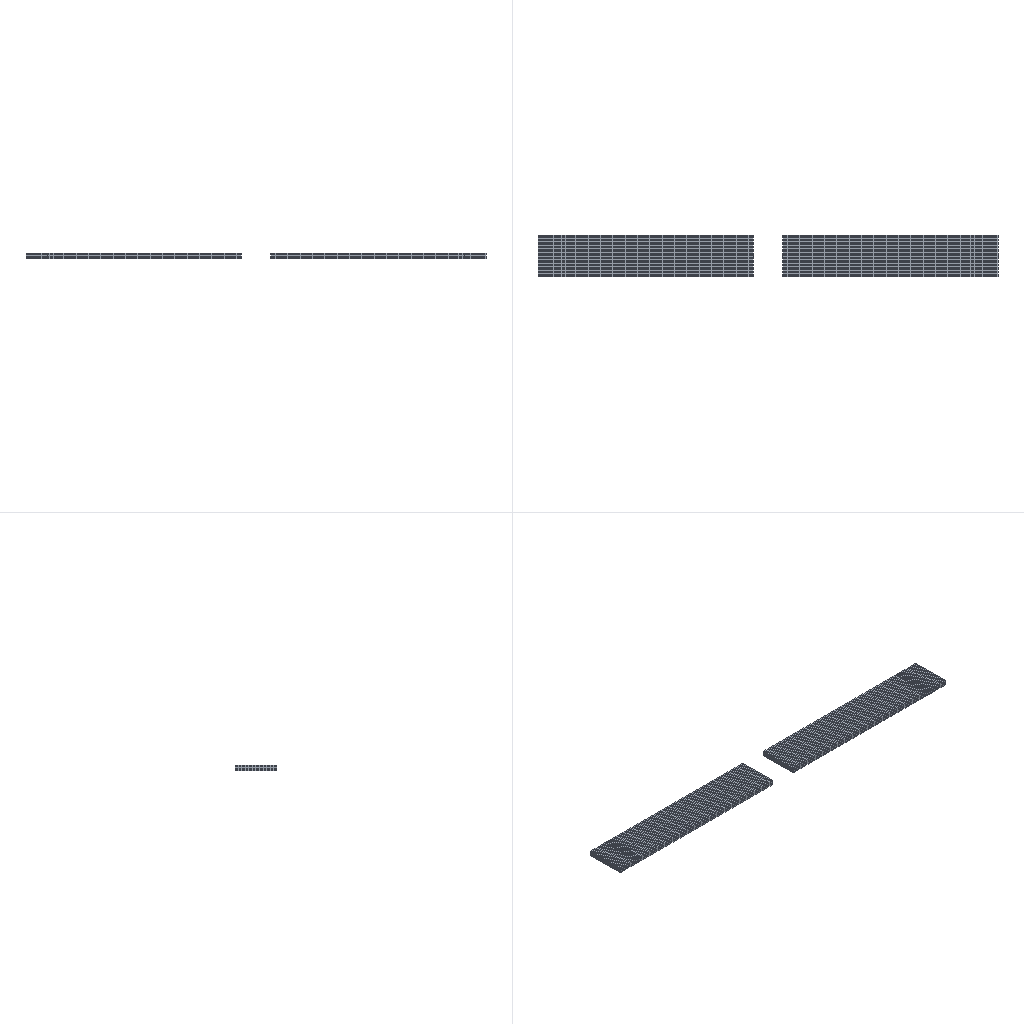Simulation study | abaqus
Set-up summary:
category,name,step,type,value,unit,region
solver,abaqus
solver,version,,,Abaqus/Explicit 2020
units,not stated in the deck,,not stated
analysis,deck,,transient,transient
load_step,Step-1,Step-1,transient
load_step,requested,,,1
mesh,nodes,,,9920
mesh,elements,,,7200
element_type,C3D8R,,solid,7200
load,load commands in deck,,count,1
bc,support commands in deck,,count,6
material,MATERIAL-1,,in results
check,setup vs results,,match,"per instance, exact: element labels, types and connectivity; labels of the nodes the elements use; coordinates not compared"
Abaqus input file, long lists of numbers shortened:
*Heading
** Job name: Job-2 Model name: Model-1-Copy
** Generated by: Abaqus/CAE 2020
*Preprint, echo=NO, model=NO, history=NO, contact=NO
**
** PARTS
**
*Part, name=Part-1
*Node
      1,           0.,           0.,           0.
      2,           0.,          -1.,           0.
** (4028 more lines like these left out)
*Element, type=C3D8R
   1,  156,  157,  188,  187,    1,    2,   33,   32
   2,  157,  158,  189,  188,    2,    3,   34,   33
** (2998 more lines like these left out)
*Nset, nset=Set-6, generate
    1,  4030,     1
*Elset, elset=Set-6, generate
    1,  3000,     1
** Section: Section-1
*Solid Section, elset=Set-6, material=Material-1
,
*End Part
**
*Part, name=Part-2
*Node
      1,           0.,         -30.,           4.
      2,           0.,         -29.,           4.
** (928 more lines like these left out)
*Element, type=C3D8R
  1, 156, 157, 188, 187,   1,   2,  33,  32
  2, 157, 158, 189, 188,   2,   3,  34,  33
** (598 more lines like these left out)
*Nset, nset=Set-7, generate
   1,  930,    1
*Elset, elset=Set-7, generate
   1,  600,    1
** Section: Section-1
*Solid Section, elset=Set-7, material=Material-1
,
*End Part
**
**
** ASSEMBLY
**
*Assembly, name=Assembly
**
*Instance, name=Part-1-1, part=Part-1
*End Instance
**
*Instance, name=Part-2-1, part=Part-2
       -15.5,           0.,           0.
*End Instance
**
*Instance, name=Part-1-1-rad-2, part=Part-1
        300.,         -30.,           0.
        300.,         -30.,           0.,         300.,         -30.,           1.,         180.
*End Instance
**
*Instance, name=Part-2-1-rad-2, part=Part-2
       315.5,         -30.,           0.
       315.5,         -30.,           0.,        315.5,         -30.,           1.,         180.
*End Instance
**
*Node
      1,         150.,         -15.,           2.
*Node
      2,         150.,         -15.,           3.
*Node
      3,         150.,         -15.,          2.5
*Node
      4,         150.,         -13.,          2.5
*Nset, nset=Set-2
 3,
*Nset, nset=Set-3, instance=Part-1-1
    1,   31,   94,  124,  125,  155,  931,  961, 1055, 1085, 3876, 3906, 4000, 4030
*Nset, nset=Set-3, instance=Part-2-1
   1,  31, 125, 155, 156, 186, 280, 310, 621, 651, 745, 775, 776, 806, 838, 868
 900, 930
*Nset, nset=Set-3, generate
 1,  3,  1
*Nset, nset=Set-3, instance=Part-1-1-rad-2
    1,   31,   94,  124,  125,  155,  931,  961, 1055, 1085, 3876, 3906, 4000, 4030
*Nset, nset=Set-3, instance=Part-2-1-rad-2
   1,  31, 125, 155, 156, 186, 280, 310, 621, 651, 745, 775, 776, 806, 838, 868
 900, 930
*Nset, nset=Set-4, instance=Part-1-1, generate
    1,  4030,     1
*Nset, nset=Set-4, instance=Part-2-1, generate
   1,  930,    1
*Nset, nset=Set-4, instance=Part-1-1-rad-2, generate
    1,  4030,     1
*Nset, nset=Set-4, instance=Part-2-1-rad-2, generate
   1,  930,    1
*Elset, elset=Set-4, instance=Part-1-1, generate
    1,  3000,     1
*Elset, elset=Set-4, instance=Part-2-1, generate
   1,  600,    1
*Elset, elset=Set-4, instance=Part-1-1-rad-2, generate
    1,  3000,     1
*Elset, elset=Set-4, instance=Part-2-1-rad-2, generate
   1,  600,    1
*Nset, nset=Set-5, instance=Part-1-1, generate
    1,  4030,     1
*Nset, nset=Set-5, instance=Part-2-1, generate
   1,  930,    1
*Nset, nset=Set-5, instance=Part-1-1-rad-2, generate
    1,  4030,     1
*Nset, nset=Set-5, instance=Part-2-1-rad-2, generate
   1,  930,    1
*Elset, elset=Set-5, instance=Part-1-1, generate
    1,  3000,     1
*Elset, elset=Set-5, instance=Part-2-1, generate
   1,  600,    1
*Elset, elset=Set-5, instance=Part-1-1-rad-2, generate
    1,  3000,     1
*Elset, elset=Set-5, instance=Part-2-1-rad-2, generate
   1,  600,    1
*Nset, nset=m_Set-1
 3,
*Elset, elset=_Surf-8_S5, internal, instance=Part-1-1
   91,   92,   93,   94,   95,   96,   97,   98,   99,  100,  101,  102,  103,  104,  105,  106
  107,  108,  109,  110,  111,  112,  113,  114,  115,  116,  117,  118,  119,  120,  211,  212
** (45 more lines like these left out)
*Elset, elset=_Surf-8_S5, internal, instance=Part-1-1-rad-2
   91,   92,   93,   94,   95,   96,   97,   98,   99,  100,  101,  102,  103,  104,  105,  106
  107,  108,  109,  110,  111,  112,  113,  114,  115,  116,  117,  118,  119,  120,  211,  212
** (45 more lines like these left out)
*Surface, type=ELEMENT, name=Surf-8
_Surf-8_S5, S5
*Elset, elset=_Surf-11_S5, internal, instance=Part-1-1
   91,   92,   93,   94,   95,   96,   97,   98,   99,  100,  101,  102,  103,  104,  105,  106
  107,  108,  109,  110,  111,  112,  113,  114,  115,  116,  117,  118,  119,  120,  211,  212
** (45 more lines like these left out)
*Elset, elset=_Surf-11_S5, internal, instance=Part-1-1-rad-2
   91,   92,   93,   94,   95,   96,   97,   98,   99,  100,  101,  102,  103,  104,  105,  106
  107,  108,  109,  110,  111,  112,  113,  114,  115,  116,  117,  118,  119,  120,  211,  212
** (45 more lines like these left out)
*Elset, elset=_Surf-11_S3, internal, instance=Part-2-1
   1,   2,   3,   4,   5,   6,   7,   8,   9,  10,  11,  12,  13,  14,  15,  16
  17,  18,  19,  20,  21,  22,  23,  24,  25,  26,  27,  28,  29,  30, 121, 122
** (8 more lines like these left out)
*Elset, elset=_Surf-11_S3, internal, instance=Part-2-1-rad-2
   1,   2,   3,   4,   5,   6,   7,   8,   9,  10,  11,  12,  13,  14,  15,  16
  17,  18,  19,  20,  21,  22,  23,  24,  25,  26,  27,  28,  29,  30, 121, 122
** (8 more lines like these left out)
*Surface, type=ELEMENT, name=Surf-11
_Surf-11_S5, S5
_Surf-11_S3, S3
*Elset, elset=_Surf-13_S5, internal, instance=Part-1-1
   91,   92,   93,   94,   95,   96,   97,   98,   99,  100,  101,  102,  103,  104,  105,  106
  107,  108,  109,  110,  111,  112,  113,  114,  115,  116,  117,  118,  119,  120,  211,  212
** (45 more lines like these left out)
*Elset, elset=_Surf-13_S5, internal, instance=Part-2-1
  91,  92,  93,  94,  95,  96,  97,  98,  99, 100, 101, 102, 103, 104, 105, 106
 107, 108, 109, 110, 111, 112, 113, 114, 115, 116, 117, 118, 119, 120, 211, 212
** (8 more lines like these left out)
*Elset, elset=_Surf-13_S5, internal, instance=Part-1-1-rad-2
   91,   92,   93,   94,   95,   96,   97,   98,   99,  100,  101,  102,  103,  104,  105,  106
  107,  108,  109,  110,  111,  112,  113,  114,  115,  116,  117,  118,  119,  120,  211,  212
** (45 more lines like these left out)
*Elset, elset=_Surf-13_S5, internal, instance=Part-2-1-rad-2
  91,  92,  93,  94,  95,  96,  97,  98,  99, 100, 101, 102, 103, 104, 105, 106
 107, 108, 109, 110, 111, 112, 113, 114, 115, 116, 117, 118, 119, 120, 211, 212
** (8 more lines like these left out)
*Elset, elset=_Surf-13_S4, internal, instance=Part-1-1, generate
   30,  3000,    30
*Elset, elset=_Surf-13_S4, internal, instance=Part-2-1, generate
  30,  600,   30
*Elset, elset=_Surf-13_S4, internal, instance=Part-1-1-rad-2, generate
   30,  3000,    30
*Elset, elset=_Surf-13_S4, internal, instance=Part-2-1-rad-2, generate
  30,  600,   30
*Elset, elset=_Surf-13_S3, internal, instance=Part-1-1
    1,    2,    3,    4,    5,    6,    7,    8,    9,   10,   11,   12,   13,   14,   15,   16
   17,   18,   19,   20,   21,   22,   23,   24,   25,   26,   27,   28,   29,   30,  121,  122
** (45 more lines like these left out)
*Elset, elset=_Surf-13_S3, internal, instance=Part-2-1
   1,   2,   3,   4,   5,   6,   7,   8,   9,  10,  11,  12,  13,  14,  15,  16
  17,  18,  19,  20,  21,  22,  23,  24,  25,  26,  27,  28,  29,  30, 121, 122
** (8 more lines like these left out)
*Elset, elset=_Surf-13_S3, internal, instance=Part-1-1-rad-2
    1,    2,    3,    4,    5,    6,    7,    8,    9,   10,   11,   12,   13,   14,   15,   16
   17,   18,   19,   20,   21,   22,   23,   24,   25,   26,   27,   28,   29,   30,  121,  122
** (45 more lines like these left out)
*Elset, elset=_Surf-13_S3, internal, instance=Part-2-1-rad-2
   1,   2,   3,   4,   5,   6,   7,   8,   9,  10,  11,  12,  13,  14,  15,  16
  17,  18,  19,  20,  21,  22,  23,  24,  25,  26,  27,  28,  29,  30, 121, 122
** (8 more lines like these left out)
*Elset, elset=_Surf-13_S6, internal, instance=Part-1-1, generate
    1,  2971,    30
*Elset, elset=_Surf-13_S6, internal, instance=Part-2-1, generate
   1,  571,   30
*Elset, elset=_Surf-13_S6, internal, instance=Part-1-1-rad-2, generate
    1,  2971,    30
*Elset, elset=_Surf-13_S6, internal, instance=Part-2-1-rad-2, generate
   1,  571,   30
*Elset, elset=_Surf-13_S2, internal, instance=Part-1-1, generate
   1,  120,    1
*Elset, elset=_Surf-13_S2, internal, instance=Part-2-1, generate
   1,  120,    1
*Elset, elset=_Surf-13_S2, internal, instance=Part-1-1-rad-2, generate
   1,  120,    1
*Elset, elset=_Surf-13_S2, internal, instance=Part-2-1-rad-2, generate
   1,  120,    1
*Elset, elset=_Surf-13_S1, internal, instance=Part-1-1, generate
 2881,  3000,     1
*Elset, elset=_Surf-13_S1, internal, instance=Part-2-1, generate
 481,  600,    1
*Elset, elset=_Surf-13_S1, internal, instance=Part-1-1-rad-2, generate
 2881,  3000,     1
*Elset, elset=_Surf-13_S1, internal, instance=Part-2-1-rad-2, generate
 481,  600,    1
*Surface, type=ELEMENT, name=Surf-13
_Surf-13_S5, S5
_Surf-13_S4, S4
_Surf-13_S6, S6
_Surf-13_S2, S2
_Surf-13_S3, S3
_Surf-13_S1, S1
*Elset, elset=_Surf-14_S2, internal, instance=Part-2-1, generate
   1,  120,    1
*Elset, elset=_Surf-14_S2, internal, instance=Part-2-1-rad-2, generate
   1,  120,    1
*Surface, type=ELEMENT, name=Surf-14
_Surf-14_S2, S2
*Elset, elset=_Surf-15_S5, internal, instance=Part-1-1
   91,   92,   93,   94,   95,   96,   97,   98,   99,  100,  101,  102,  103,  104,  105,  106
  107,  108,  109,  110,  111,  112,  113,  114,  115,  116,  117,  118,  119,  120,  211,  212
** (45 more lines like these left out)
*Elset, elset=_Surf-15_S5, internal, instance=Part-1-1-rad-2
   91,   92,   93,   94,   95,   96,   97,   98,   99,  100,  101,  102,  103,  104,  105,  106
  107,  108,  109,  110,  111,  112,  113,  114,  115,  116,  117,  118,  119,  120,  211,  212
** (45 more lines like these left out)
*Elset, elset=_Surf-15_S3, internal, instance=Part-2-1
   1,   2,   3,   4,   5,   6,   7,   8,   9,  10,  11,  12,  13,  14,  15,  16
  17,  18,  19,  20,  21,  22,  23,  24,  25,  26,  27,  28,  29,  30, 121, 122
** (8 more lines like these left out)
*Elset, elset=_Surf-15_S3, internal, instance=Part-2-1-rad-2
   1,   2,   3,   4,   5,   6,   7,   8,   9,  10,  11,  12,  13,  14,  15,  16
  17,  18,  19,  20,  21,  22,  23,  24,  25,  26,  27,  28,  29,  30, 121, 122
** (8 more lines like these left out)
*Surface, type=ELEMENT, name=Surf-15
_Surf-15_S5, S5
_Surf-15_S3, S3
*Elset, elset=_Surf-16_S5, internal, instance=Part-1-1
   91,   92,   93,   94,   95,   96,   97,   98,   99,  100,  101,  102,  103,  104,  105,  106
  107,  108,  109,  110,  111,  112,  113,  114,  115,  116,  117,  118,  119,  120,  211,  212
** (45 more lines like these left out)
*Elset, elset=_Surf-16_S5, internal, instance=Part-2-1-rad-2
  91,  92,  93,  94,  95,  96,  97,  98,  99, 100, 101, 102, 103, 104, 105, 106
 107, 108, 109, 110, 111, 112, 113, 114, 115, 116, 117, 118, 119, 120, 211, 212
** (8 more lines like these left out)
*Elset, elset=_Surf-16_S3, internal, instance=Part-2-1
   1,   2,   3,   4,   5,   6,   7,   8,   9,  10,  11,  12,  13,  14,  15,  16
  17,  18,  19,  20,  21,  22,  23,  24,  25,  26,  27,  28,  29,  30, 121, 122
** (8 more lines like these left out)
*Elset, elset=_Surf-16_S3, internal, instance=Part-1-1-rad-2
    1,    2,    3,    4,    5,    6,    7,    8,    9,   10,   11,   12,   13,   14,   15,   16
   17,   18,   19,   20,   21,   22,   23,   24,   25,   26,   27,   28,   29,   30,  121,  122
** (45 more lines like these left out)
*Surface, type=ELEMENT, name=Surf-16
_Surf-16_S5, S5
_Surf-16_S3, S3
*Elset, elset=_Surf-17_S3, internal, instance=Part-1-1
    1,    2,    3,    4,    5,    6,    7,    8,    9,   10,   11,   12,   13,   14,   15,   16
   17,   18,   19,   20,   21,   22,   23,   24,   25,   26,   27,   28,   29,   30,  121,  122
** (45 more lines like these left out)
*Elset, elset=_Surf-17_S3, internal, instance=Part-2-1-rad-2
   1,   2,   3,   4,   5,   6,   7,   8,   9,  10,  11,  12,  13,  14,  15,  16
  17,  18,  19,  20,  21,  22,  23,  24,  25,  26,  27,  28,  29,  30, 121, 122
** (8 more lines like these left out)
*Elset, elset=_Surf-17_S5, internal, instance=Part-2-1
  91,  92,  93,  94,  95,  96,  97,  98,  99, 100, 101, 102, 103, 104, 105, 106
 107, 108, 109, 110, 111, 112, 113, 114, 115, 116, 117, 118, 119, 120, 211, 212
** (8 more lines like these left out)
*Elset, elset=_Surf-17_S5, internal, instance=Part-1-1-rad-2
   91,   92,   93,   94,   95,   96,   97,   98,   99,  100,  101,  102,  103,  104,  105,  106
  107,  108,  109,  110,  111,  112,  113,  114,  115,  116,  117,  118,  119,  120,  211,  212
** (45 more lines like these left out)
*Surface, type=ELEMENT, name=Surf-17
_Surf-17_S3, S3
_Surf-17_S5, S5
*Elset, elset=_Surf-18_S5, internal, instance=Part-1-1
   91,   92,   93,   94,   95,   96,   97,   98,   99,  100,  101,  102,  103,  104,  105,  106
  107,  108,  109,  110,  111,  112,  113,  114,  115,  116,  117,  118,  119,  120,  211,  212
** (45 more lines like these left out)
*Elset, elset=_Surf-18_S5, internal, instance=Part-1-1-rad-2
   91,   92,   93,   94,   95,   96,   97,   98,   99,  100,  101,  102,  103,  104,  105,  106
  107,  108,  109,  110,  111,  112,  113,  114,  115,  116,  117,  118,  119,  120,  211,  212
** (45 more lines like these left out)
*Elset, elset=_Surf-18_S3, internal, instance=Part-2-1
   1,   2,   3,   4,   5,   6,   7,   8,   9,  10,  11,  12,  13,  14,  15,  16
  17,  18,  19,  20,  21,  22,  23,  24,  25,  26,  27,  28,  29,  30, 121, 122
** (8 more lines like these left out)
*Elset, elset=_Surf-18_S3, internal, instance=Part-2-1-rad-2
   1,   2,   3,   4,   5,   6,   7,   8,   9,  10,  11,  12,  13,  14,  15,  16
  17,  18,  19,  20,  21,  22,  23,  24,  25,  26,  27,  28,  29,  30, 121, 122
** (8 more lines like these left out)
*Surface, type=ELEMENT, name=Surf-18
_Surf-18_S5, S5
_Surf-18_S3, S3
*Elset, elset=_m_Surf-1_S2, internal, instance=Part-1-1, generate
  1,  90,   1
*Surface, type=ELEMENT, name=m_Surf-1
_m_Surf-1_S2, S2
*Elset, elset=_m_Surf-5_S2, internal, instance=Part-1-1-rad-2, generate
   1,  120,    1
*Surface, type=ELEMENT, name=m_Surf-5
_m_Surf-5_S2, S2
*Elset, elset=_s_Surf-3_S2, internal, instance=Part-1-1, generate
  91,  120,    1
*Surface, type=ELEMENT, name=s_Surf-3
_s_Surf-3_S2, S2
*Elset, elset=_s_Surf-7_S1, internal, instance=Part-1-1, generate
 2881,  3000,     1
*Elset, elset=_s_Surf-7_S1, internal, instance=Part-1-1-rad-2, generate
 2881,  3000,     1
*Surface, type=ELEMENT, name=s_Surf-7
_s_Surf-7_S1, S1
*Elset, elset=_s_Surf-9_S1, internal, instance=Part-2-1, generate
 541,  600,    1
*Surface, type=ELEMENT, name=s_Surf-9
_s_Surf-9_S1, S1
*Elset, elset=_s_Surf-10_S1, internal, instance=Part-2-1-rad-2, generate
 481,  600,    1
*Surface, type=ELEMENT, name=s_Surf-10
_s_Surf-10_S1, S1
*Elset, elset=_s_Surf-12_S1, internal, instance=Part-2-1, generate
 481,  540,    1
*Surface, type=ELEMENT, name=s_Surf-12
_s_Surf-12_S1, S1
** Constraint: Constraint-1
*Tie, name=Constraint-1, adjust=yes
s_Surf-9, m_Surf-1
** Constraint: Constraint-2
*Tie, name=Constraint-2, adjust=yes
s_Surf-10, m_Surf-5
** Constraint: Constraint-3
*Coupling, constraint name=Constraint-3, ref node=m_Set-1, surface=s_Surf-7
*Kinematic
*Nonstructural Mass, elset=Set-4, units=MASS PER VOLUME
7.8e-09,
*End Assembly
*Amplitude, name=Amp-1, definition=PERIODIC
1,           2093.,              0.,              0.
             1.,              0.
*Amplitude, name=Amp-2, definition=PERIODIC
1,            628.,              0.,              0.
             1.,              0.
**
** MATERIALS
**
*Material, name=Material-1
*Density
 7.8e-09,
*Elastic
210000., 0.3
**
** INTERACTION PROPERTIES
**
*Surface Interaction, name=IntProp-1
*Friction
 0.2,
*Surface Behavior, pressure-overclosure=HARD
** ----------------------------------------------------------------
**
** STEP: Step-1
**
*Step, name=Step-1, nlgeom=YES
*Dynamic, Explicit
, 0.015
*Bulk Viscosity
0.06, 1.2
**
** BOUNDARY CONDITIONS
**
** Name: BC-1 Type: 速度/角速度
*Boundary, amplitude=Amp-1, type=VELOCITY
Set-2, 1, 1
Set-2, 2, 2
Set-2, 3, 3
Set-2, 4, 4
Set-2, 5, 5, 2094.
Set-2, 6, 6
**
** INTERACTIONS
**
** Interaction: Int-1
*Contact Pair, interaction=IntProp-1, mechanical constraint=KINEMATIC, cpset=Int-1
s_Surf-3, s_Surf-12
**
** OUTPUT REQUESTS
**
*Restart, write, number interval=1, time marks=NO
**
** FIELD OUTPUT: F-Output-1
**
*Output, field, number interval=500
*Node Output
A, RF, U, V
*Element Output, directions=YES
E, LE, MISES, PE, PEEQ, S
*Contact Output
CSTRESS,
**
** HISTORY OUTPUT: H-Output-1
**
*Output, history, variable=PRESELECT
*End Step
Results summary:
result,step,Step-1,completed,increments=86757 time=0.015/0.015
result,analysis,,,transient
result,last_loadstep,,,1
result,primary field,,,U
result,reaction total,,FX,28609.109,model units
result,reaction total,,FY,-199352.594,model units
result,reaction total,,FZ,28562.102,model units